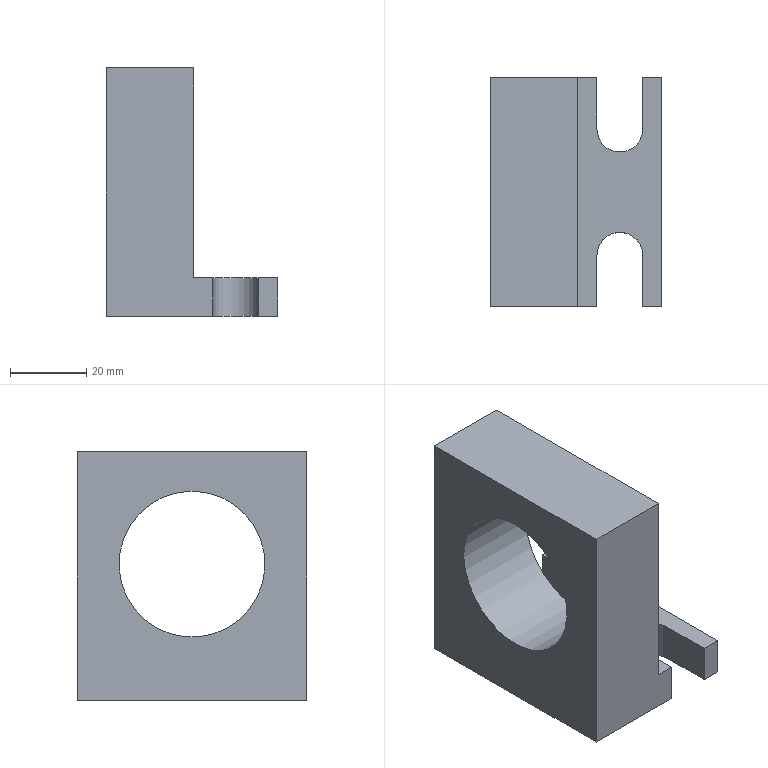Part | NX | features solid 2 | 1 solid | 17 faces | box 45 x 60 x 65 mm | volume 72169 mm3 | plane 14 | cylinder 3 | commonest cylinder face diameters 12 x2 38.2 x1
STEP:
#1=CARTESIAN_POINT('',(350.,-180.,-430.3));
#2=VERTEX_POINT('',#1);
#3=CARTESIAN_POINT('',(350.,-180.,-449.4));
#4=DIRECTION('',(-1.,0.,0.));
#5=DIRECTION('',(0.,0.,1.));
#6=AXIS2_PLACEMENT_3D('',#3,#4,#5);
#7=CIRCLE('',#6,19.1);
#8=EDGE_CURVE('',#2,#2,#7,.T.);
#9=ORIENTED_EDGE('',*,*,#8,.F.);
#10=EDGE_LOOP('',(#9));
#11=FACE_BOUND('',#10,.T.);
#12=CARTESIAN_POINT('',(350.,-150.,-420.));
#13=VERTEX_POINT('',#12);
#14=CARTESIAN_POINT('',(350.,-150.,-485.));
#15=VERTEX_POINT('',#14);
#16=CARTESIAN_POINT('',(350.,-150.,-417.4));
#17=DIRECTION('',(0.,0.,-1.));
#18=VECTOR('',#17,1000.);
#19=LINE('',#16,#18);
#20=EDGE_CURVE('',#13,#15,#19,.T.);
#21=ORIENTED_EDGE('',*,*,#20,.T.);
#22=CARTESIAN_POINT('',(350.,-210.,-485.));
#23=VERTEX_POINT('',#22);
#24=CARTESIAN_POINT('',(350.,-212.5,-485.));
#25=DIRECTION('',(0.,-1.,0.));
#26=VECTOR('',#25,1000.);
#27=LINE('',#24,#26);
#28=EDGE_CURVE('',#23,#15,#27,.F.);
#29=ORIENTED_EDGE('',*,*,#28,.F.);
#30=CARTESIAN_POINT('',(350.,-210.,-420.));
#31=VERTEX_POINT('',#30);
#32=CARTESIAN_POINT('',(350.,-210.,-417.4));
#33=DIRECTION('',(0.,0.,1.));
#34=VECTOR('',#33,1000.);
#35=LINE('',#32,#34);
#36=EDGE_CURVE('',#31,#23,#35,.F.);
#37=ORIENTED_EDGE('',*,*,#36,.F.);
#38=CARTESIAN_POINT('',(350.,-212.5,-420.));
#39=DIRECTION('',(0.,1.,0.));
#40=VECTOR('',#39,1000.);
#41=LINE('',#38,#40);
#42=EDGE_CURVE('',#31,#13,#41,.T.);
#43=ORIENTED_EDGE('',*,*,#42,.T.);
#44=EDGE_LOOP('',(#21,#29,#37,#43));
#45=FACE_BOUND('',#44,.T.);
#46=CARTESIAN_POINT('',(350.,-212.5,-417.4));
#47=DIRECTION('',(-1.,0.,0.));
#48=DIRECTION('',(0.,0.,-1.));
#49=AXIS2_PLACEMENT_3D('',#46,#47,#48);
#50=PLANE('',#49);
#51=ADVANCED_FACE('',(#11,#45),#50,.T.);
#52=CARTESIAN_POINT('',(395.,-210.,-485.));
#53=VERTEX_POINT('',#52);
#54=CARTESIAN_POINT('',(395.,-150.,-485.));
#55=VERTEX_POINT('',#54);
#56=CARTESIAN_POINT('',(395.,-212.5,-485.));
#57=DIRECTION('',(0.,-1.,0.));
#58=VECTOR('',#57,1000.);
#59=LINE('',#56,#58);
#60=EDGE_CURVE('',#53,#55,#59,.F.);
#61=ORIENTED_EDGE('',*,*,#60,.T.);
#62=CARTESIAN_POINT('',(395.,-150.,-475.));
#63=VERTEX_POINT('',#62);
#64=CARTESIAN_POINT('',(395.,-150.,-417.4));
#65=DIRECTION('',(0.,0.,-1.));
#66=VECTOR('',#65,1000.);
#67=LINE('',#64,#66);
#68=EDGE_CURVE('',#63,#55,#67,.T.);
#69=ORIENTED_EDGE('',*,*,#68,.F.);
#70=CARTESIAN_POINT('',(395.,-210.,-475.));
#71=VERTEX_POINT('',#70);
#72=CARTESIAN_POINT('',(395.,-212.5,-475.));
#73=DIRECTION('',(0.,1.,0.));
#74=VECTOR('',#73,1000.);
#75=LINE('',#72,#74);
#76=EDGE_CURVE('',#71,#63,#75,.T.);
#77=ORIENTED_EDGE('',*,*,#76,.F.);
#78=CARTESIAN_POINT('',(395.,-210.,-487.4));
#79=DIRECTION('',(0.,0.,1.));
#80=VECTOR('',#79,1000.);
#81=LINE('',#78,#80);
#82=EDGE_CURVE('',#71,#53,#81,.F.);
#83=ORIENTED_EDGE('',*,*,#82,.T.);
#84=EDGE_LOOP('',(#61,#69,#77,#83));
#85=FACE_BOUND('',#84,.T.);
#86=CARTESIAN_POINT('',(395.,-212.5,-487.4));
#87=DIRECTION('',(-1.,0.,0.));
#88=DIRECTION('',(0.,1.,0.));
#89=AXIS2_PLACEMENT_3D('',#86,#87,#88);
#90=PLANE('',#89);
#91=ADVANCED_FACE('',(#85),#90,.F.);
#92=CARTESIAN_POINT('',(378.,-210.,-485.));
#93=VERTEX_POINT('',#92);
#94=CARTESIAN_POINT('',(378.,-210.,-475.));
#95=VERTEX_POINT('',#94);
#96=CARTESIAN_POINT('',(378.,-210.,-524.4));
#97=DIRECTION('',(0.,0.,-1.));
#98=VECTOR('',#97,1000.);
#99=LINE('',#96,#98);
#100=EDGE_CURVE('',#93,#95,#99,.F.);
#101=ORIENTED_EDGE('',*,*,#100,.T.);
#102=CARTESIAN_POINT('',(373.,-210.,-475.));
#103=VERTEX_POINT('',#102);
#104=CARTESIAN_POINT('',(373.,-210.,-475.));
#105=DIRECTION('',(-1.,0.,0.));
#106=VECTOR('',#105,1000.);
#107=LINE('',#104,#106);
#108=EDGE_CURVE('',#103,#95,#107,.F.);
#109=ORIENTED_EDGE('',*,*,#108,.F.);
#110=CARTESIAN_POINT('',(373.,-210.,-420.));
#111=VERTEX_POINT('',#110);
#112=CARTESIAN_POINT('',(373.,-210.,-417.4));
#113=DIRECTION('',(0.,0.,1.));
#114=VECTOR('',#113,1000.);
#115=LINE('',#112,#114);
#116=EDGE_CURVE('',#111,#103,#115,.F.);
#117=ORIENTED_EDGE('',*,*,#116,.F.);
#118=CARTESIAN_POINT('',(373.,-210.,-420.));
#119=DIRECTION('',(-1.,0.,0.));
#120=VECTOR('',#119,1000.);
#121=LINE('',#118,#120);
#122=EDGE_CURVE('',#31,#111,#121,.F.);
#123=ORIENTED_EDGE('',*,*,#122,.F.);
#124=ORIENTED_EDGE('',*,*,#36,.T.);
#125=CARTESIAN_POINT('',(373.,-210.,-485.));
#126=DIRECTION('',(1.,0.,0.));
#127=VECTOR('',#126,1000.);
#128=LINE('',#125,#127);
#129=EDGE_CURVE('',#23,#93,#128,.T.);
#130=ORIENTED_EDGE('',*,*,#129,.T.);
#131=EDGE_LOOP('',(#101,#109,#117,#123,#124,#130));
#132=FACE_BOUND('',#131,.T.);
#133=CARTESIAN_POINT('',(373.,-210.,-417.4));
#134=DIRECTION('',(0.,-1.,0.));
#135=DIRECTION('',(0.,0.,-1.));
#136=AXIS2_PLACEMENT_3D('',#133,#134,#135);
#137=PLANE('',#136);
#138=ADVANCED_FACE('',(#132),#137,.T.);
#139=ORIENTED_EDGE('',*,*,#60,.F.);
#140=CARTESIAN_POINT('',(390.,-210.,-485.));
#141=VERTEX_POINT('',#140);
#142=CARTESIAN_POINT('',(373.,-210.,-485.));
#143=DIRECTION('',(1.,0.,0.));
#144=VECTOR('',#143,1000.);
#145=LINE('',#142,#144);
#146=EDGE_CURVE('',#141,#53,#145,.T.);
#147=ORIENTED_EDGE('',*,*,#146,.F.);
#148=CARTESIAN_POINT('',(390.,-196.5,-485.));
#149=VERTEX_POINT('',#148);
#150=CARTESIAN_POINT('',(390.,-212.5,-485.));
#151=DIRECTION('',(0.,1.,0.));
#152=VECTOR('',#151,1000.);
#153=LINE('',#150,#152);
#154=EDGE_CURVE('',#149,#141,#153,.F.);
#155=ORIENTED_EDGE('',*,*,#154,.F.);
#156=CARTESIAN_POINT('',(378.,-196.5,-485.));
#157=VERTEX_POINT('',#156);
#158=CARTESIAN_POINT('',(384.,-196.5,-485.));
#159=DIRECTION('',(0.,0.,1.));
#160=DIRECTION('',(0.,1.,0.));
#161=AXIS2_PLACEMENT_3D('',#158,#159,#160);
#162=CIRCLE('',#161,6.);
#163=EDGE_CURVE('',#157,#149,#162,.F.);
#164=ORIENTED_EDGE('',*,*,#163,.F.);
#165=CARTESIAN_POINT('',(378.,-212.5,-485.));
#166=DIRECTION('',(0.,1.,0.));
#167=VECTOR('',#166,1000.);
#168=LINE('',#165,#167);
#169=EDGE_CURVE('',#157,#93,#168,.F.);
#170=ORIENTED_EDGE('',*,*,#169,.T.);
#171=ORIENTED_EDGE('',*,*,#129,.F.);
#172=ORIENTED_EDGE('',*,*,#28,.T.);
#173=CARTESIAN_POINT('',(378.,-150.,-485.));
#174=VERTEX_POINT('',#173);
#175=CARTESIAN_POINT('',(373.,-150.,-485.));
#176=DIRECTION('',(-1.,0.,0.));
#177=VECTOR('',#176,1000.);
#178=LINE('',#175,#177);
#179=EDGE_CURVE('',#15,#174,#178,.F.);
#180=ORIENTED_EDGE('',*,*,#179,.T.);
#181=CARTESIAN_POINT('',(378.,-163.5,-485.));
#182=VERTEX_POINT('',#181);
#183=CARTESIAN_POINT('',(378.,-212.5,-485.));
#184=DIRECTION('',(0.,-1.,0.));
#185=VECTOR('',#184,1000.);
#186=LINE('',#183,#185);
#187=EDGE_CURVE('',#182,#174,#186,.F.);
#188=ORIENTED_EDGE('',*,*,#187,.F.);
#189=CARTESIAN_POINT('',(390.,-163.5,-485.));
#190=VERTEX_POINT('',#189);
#191=CARTESIAN_POINT('',(384.,-163.5,-485.));
#192=DIRECTION('',(0.,0.,1.));
#193=DIRECTION('',(0.,1.,0.));
#194=AXIS2_PLACEMENT_3D('',#191,#192,#193);
#195=CIRCLE('',#194,6.);
#196=EDGE_CURVE('',#190,#182,#195,.F.);
#197=ORIENTED_EDGE('',*,*,#196,.F.);
#198=CARTESIAN_POINT('',(390.,-150.,-485.));
#199=VERTEX_POINT('',#198);
#200=CARTESIAN_POINT('',(390.,-212.5,-485.));
#201=DIRECTION('',(0.,-1.,0.));
#202=VECTOR('',#201,1000.);
#203=LINE('',#200,#202);
#204=EDGE_CURVE('',#190,#199,#203,.F.);
#205=ORIENTED_EDGE('',*,*,#204,.T.);
#206=CARTESIAN_POINT('',(373.,-150.,-485.));
#207=DIRECTION('',(-1.,0.,0.));
#208=VECTOR('',#207,1000.);
#209=LINE('',#206,#208);
#210=EDGE_CURVE('',#199,#55,#209,.F.);
#211=ORIENTED_EDGE('',*,*,#210,.T.);
#212=EDGE_LOOP('',(#139,#147,#155,#164,#170,#171,#172,#180,#188,#197,#205,#211));
#213=FACE_BOUND('',#212,.T.);
#214=CARTESIAN_POINT('',(373.,-212.5,-485.));
#215=DIRECTION('',(0.,0.,-1.));
#216=DIRECTION('',(0.,1.,0.));
#217=AXIS2_PLACEMENT_3D('',#214,#215,#216);
#218=PLANE('',#217);
#219=ADVANCED_FACE('',(#213),#218,.T.);
#220=CARTESIAN_POINT('',(378.,-196.5,-475.));
#221=VERTEX_POINT('',#220);
#222=CARTESIAN_POINT('',(390.,-196.5,-475.));
#223=VERTEX_POINT('',#222);
#224=CARTESIAN_POINT('',(384.,-196.5,-475.));
#225=DIRECTION('',(0.,0.,-1.));
#226=DIRECTION('',(0.,-1.,0.));
#227=AXIS2_PLACEMENT_3D('',#224,#225,#226);
#228=CIRCLE('',#227,6.);
#229=EDGE_CURVE('',#221,#223,#228,.T.);
#230=ORIENTED_EDGE('',*,*,#229,.T.);
#231=CARTESIAN_POINT('',(390.,-210.,-475.));
#232=VERTEX_POINT('',#231);
#233=CARTESIAN_POINT('',(390.,-212.5,-475.));
#234=DIRECTION('',(0.,-1.,0.));
#235=VECTOR('',#234,1000.);
#236=LINE('',#233,#235);
#237=EDGE_CURVE('',#223,#232,#236,.T.);
#238=ORIENTED_EDGE('',*,*,#237,.T.);
#239=CARTESIAN_POINT('',(373.,-210.,-475.));
#240=DIRECTION('',(-1.,0.,0.));
#241=VECTOR('',#240,1000.);
#242=LINE('',#239,#241);
#243=EDGE_CURVE('',#232,#71,#242,.F.);
#244=ORIENTED_EDGE('',*,*,#243,.T.);
#245=ORIENTED_EDGE('',*,*,#76,.T.);
#246=CARTESIAN_POINT('',(390.,-150.,-475.));
#247=VERTEX_POINT('',#246);
#248=CARTESIAN_POINT('',(373.,-150.,-475.));
#249=DIRECTION('',(1.,0.,0.));
#250=VECTOR('',#249,1000.);
#251=LINE('',#248,#250);
#252=EDGE_CURVE('',#247,#63,#251,.T.);
#253=ORIENTED_EDGE('',*,*,#252,.F.);
#254=CARTESIAN_POINT('',(390.,-163.5,-475.));
#255=VERTEX_POINT('',#254);
#256=CARTESIAN_POINT('',(390.,-212.5,-475.));
#257=DIRECTION('',(0.,1.,0.));
#258=VECTOR('',#257,1000.);
#259=LINE('',#256,#258);
#260=EDGE_CURVE('',#255,#247,#259,.T.);
#261=ORIENTED_EDGE('',*,*,#260,.F.);
#262=CARTESIAN_POINT('',(378.,-163.5,-475.));
#263=VERTEX_POINT('',#262);
#264=CARTESIAN_POINT('',(384.,-163.5,-475.));
#265=DIRECTION('',(0.,0.,-1.));
#266=DIRECTION('',(0.,-1.,0.));
#267=AXIS2_PLACEMENT_3D('',#264,#265,#266);
#268=CIRCLE('',#267,6.);
#269=EDGE_CURVE('',#255,#263,#268,.T.);
#270=ORIENTED_EDGE('',*,*,#269,.T.);
#271=CARTESIAN_POINT('',(378.,-150.,-475.));
#272=VERTEX_POINT('',#271);
#273=CARTESIAN_POINT('',(378.,-212.5,-475.));
#274=DIRECTION('',(0.,1.,0.));
#275=VECTOR('',#274,1000.);
#276=LINE('',#273,#275);
#277=EDGE_CURVE('',#263,#272,#276,.T.);
#278=ORIENTED_EDGE('',*,*,#277,.T.);
#279=CARTESIAN_POINT('',(373.,-150.,-475.));
#280=VERTEX_POINT('',#279);
#281=CARTESIAN_POINT('',(373.,-150.,-475.));
#282=DIRECTION('',(1.,0.,0.));
#283=VECTOR('',#282,1000.);
#284=LINE('',#281,#283);
#285=EDGE_CURVE('',#280,#272,#284,.T.);
#286=ORIENTED_EDGE('',*,*,#285,.F.);
#287=CARTESIAN_POINT('',(373.,-212.5,-475.));
#288=DIRECTION('',(0.,1.,0.));
#289=VECTOR('',#288,1000.);
#290=LINE('',#287,#289);
#291=EDGE_CURVE('',#103,#280,#290,.T.);
#292=ORIENTED_EDGE('',*,*,#291,.F.);
#293=ORIENTED_EDGE('',*,*,#108,.T.);
#294=CARTESIAN_POINT('',(378.,-212.5,-475.));
#295=DIRECTION('',(0.,-1.,0.));
#296=VECTOR('',#295,1000.);
#297=LINE('',#294,#296);
#298=EDGE_CURVE('',#221,#95,#297,.T.);
#299=ORIENTED_EDGE('',*,*,#298,.F.);
#300=EDGE_LOOP('',(#230,#238,#244,#245,#253,#261,#270,#278,#286,#292,#293,#299));
#301=FACE_BOUND('',#300,.T.);
#302=CARTESIAN_POINT('',(373.,-212.5,-475.));
#303=DIRECTION('',(0.,0.,1.));
#304=DIRECTION('',(-1.,0.,0.));
#305=AXIS2_PLACEMENT_3D('',#302,#303,#304);
#306=PLANE('',#305);
#307=ADVANCED_FACE('',(#301),#306,.T.);
#308=CARTESIAN_POINT('',(390.,-150.,-524.4));
#309=DIRECTION('',(0.,0.,1.));
#310=VECTOR('',#309,1000.);
#311=LINE('',#308,#310);
#312=EDGE_CURVE('',#199,#247,#311,.T.);
#313=ORIENTED_EDGE('',*,*,#312,.T.);
#314=ORIENTED_EDGE('',*,*,#252,.T.);
#315=ORIENTED_EDGE('',*,*,#68,.T.);
#316=ORIENTED_EDGE('',*,*,#210,.F.);
#317=EDGE_LOOP('',(#313,#314,#315,#316));
#318=FACE_BOUND('',#317,.T.);
#319=CARTESIAN_POINT('',(373.,-150.,-417.4));
#320=DIRECTION('',(0.,-1.,0.));
#321=DIRECTION('',(0.,0.,-1.));
#322=AXIS2_PLACEMENT_3D('',#319,#320,#321);
#323=PLANE('',#322);
#324=ADVANCED_FACE('',(#318),#323,.F.);
#325=ORIENTED_EDGE('',*,*,#116,.T.);
#326=ORIENTED_EDGE('',*,*,#291,.T.);
#327=CARTESIAN_POINT('',(373.,-150.,-420.));
#328=VERTEX_POINT('',#327);
#329=CARTESIAN_POINT('',(373.,-150.,-417.4));
#330=DIRECTION('',(0.,0.,-1.));
#331=VECTOR('',#330,1000.);
#332=LINE('',#329,#331);
#333=EDGE_CURVE('',#328,#280,#332,.T.);
#334=ORIENTED_EDGE('',*,*,#333,.F.);
#335=CARTESIAN_POINT('',(373.,-212.5,-420.));
#336=DIRECTION('',(0.,1.,0.));
#337=VECTOR('',#336,1000.);
#338=LINE('',#335,#337);
#339=EDGE_CURVE('',#111,#328,#338,.T.);
#340=ORIENTED_EDGE('',*,*,#339,.F.);
#341=EDGE_LOOP('',(#325,#326,#334,#340));
#342=FACE_BOUND('',#341,.T.);
#343=CARTESIAN_POINT('',(373.,-180.,-430.3));
#344=VERTEX_POINT('',#343);
#345=CARTESIAN_POINT('',(373.,-180.,-449.4));
#346=DIRECTION('',(-1.,0.,0.));
#347=DIRECTION('',(0.,0.,1.));
#348=AXIS2_PLACEMENT_3D('',#345,#346,#347);
#349=CIRCLE('',#348,19.1);
#350=EDGE_CURVE('',#344,#344,#349,.F.);
#351=ORIENTED_EDGE('',*,*,#350,.F.);
#352=EDGE_LOOP('',(#351));
#353=FACE_BOUND('',#352,.T.);
#354=CARTESIAN_POINT('',(373.,-212.5,-417.4));
#355=DIRECTION('',(-1.,0.,0.));
#356=DIRECTION('',(0.,0.,-1.));
#357=AXIS2_PLACEMENT_3D('',#354,#355,#356);
#358=PLANE('',#357);
#359=ADVANCED_FACE('',(#342,#353),#358,.F.);
#360=ORIENTED_EDGE('',*,*,#146,.T.);
#361=ORIENTED_EDGE('',*,*,#82,.F.);
#362=ORIENTED_EDGE('',*,*,#243,.F.);
#363=CARTESIAN_POINT('',(390.,-210.,-524.4));
#364=DIRECTION('',(0.,0.,-1.));
#365=VECTOR('',#364,1000.);
#366=LINE('',#363,#365);
#367=EDGE_CURVE('',#141,#232,#366,.F.);
#368=ORIENTED_EDGE('',*,*,#367,.F.);
#369=EDGE_LOOP('',(#360,#361,#362,#368));
#370=FACE_BOUND('',#369,.T.);
#371=CARTESIAN_POINT('',(373.,-210.,-417.4));
#372=DIRECTION('',(0.,-1.,0.));
#373=DIRECTION('',(0.,0.,-1.));
#374=AXIS2_PLACEMENT_3D('',#371,#372,#373);
#375=PLANE('',#374);
#376=ADVANCED_FACE('',(#370),#375,.T.);
#377=ORIENTED_EDGE('',*,*,#179,.F.);
#378=ORIENTED_EDGE('',*,*,#20,.F.);
#379=CARTESIAN_POINT('',(373.,-150.,-420.));
#380=DIRECTION('',(1.,0.,0.));
#381=VECTOR('',#380,1000.);
#382=LINE('',#379,#381);
#383=EDGE_CURVE('',#13,#328,#382,.T.);
#384=ORIENTED_EDGE('',*,*,#383,.T.);
#385=ORIENTED_EDGE('',*,*,#333,.T.);
#386=ORIENTED_EDGE('',*,*,#285,.T.);
#387=CARTESIAN_POINT('',(378.,-150.,-524.4));
#388=DIRECTION('',(0.,0.,1.));
#389=VECTOR('',#388,1000.);
#390=LINE('',#387,#389);
#391=EDGE_CURVE('',#174,#272,#390,.T.);
#392=ORIENTED_EDGE('',*,*,#391,.F.);
#393=EDGE_LOOP('',(#377,#378,#384,#385,#386,#392));
#394=FACE_BOUND('',#393,.T.);
#395=CARTESIAN_POINT('',(373.,-150.,-417.4));
#396=DIRECTION('',(0.,-1.,0.));
#397=DIRECTION('',(0.,0.,-1.));
#398=AXIS2_PLACEMENT_3D('',#395,#396,#397);
#399=PLANE('',#398);
#400=ADVANCED_FACE('',(#394),#399,.F.);
#401=ORIENTED_EDGE('',*,*,#42,.F.);
#402=ORIENTED_EDGE('',*,*,#122,.T.);
#403=ORIENTED_EDGE('',*,*,#339,.T.);
#404=ORIENTED_EDGE('',*,*,#383,.F.);
#405=EDGE_LOOP('',(#401,#402,#403,#404));
#406=FACE_BOUND('',#405,.T.);
#407=CARTESIAN_POINT('',(373.,-212.5,-420.));
#408=DIRECTION('',(0.,0.,-1.));
#409=DIRECTION('',(0.,1.,0.));
#410=AXIS2_PLACEMENT_3D('',#407,#408,#409);
#411=PLANE('',#410);
#412=ADVANCED_FACE('',(#406),#411,.F.);
#413=ORIENTED_EDGE('',*,*,#8,.T.);
#414=EDGE_LOOP('',(#413));
#415=FACE_BOUND('',#414,.T.);
#416=ORIENTED_EDGE('',*,*,#350,.T.);
#417=EDGE_LOOP('',(#416));
#418=FACE_BOUND('',#417,.T.);
#419=CARTESIAN_POINT('',(293.,-180.,-449.4));
#420=DIRECTION('',(1.,0.,0.));
#421=DIRECTION('',(0.,0.,1.));
#422=AXIS2_PLACEMENT_3D('',#419,#420,#421);
#423=CYLINDRICAL_SURFACE('',#422,19.1);
#424=ADVANCED_FACE('',(#415,#418),#423,.F.);
#425=CARTESIAN_POINT('',(378.,-163.5,-524.4));
#426=DIRECTION('',(0.,0.,1.));
#427=VECTOR('',#426,1000.);
#428=LINE('',#425,#427);
#429=EDGE_CURVE('',#182,#263,#428,.T.);
#430=ORIENTED_EDGE('',*,*,#429,.F.);
#431=ORIENTED_EDGE('',*,*,#187,.T.);
#432=ORIENTED_EDGE('',*,*,#391,.T.);
#433=ORIENTED_EDGE('',*,*,#277,.F.);
#434=EDGE_LOOP('',(#430,#431,#432,#433));
#435=FACE_BOUND('',#434,.T.);
#436=CARTESIAN_POINT('',(378.,-163.5,-524.4));
#437=DIRECTION('',(-1.,0.,0.));
#438=DIRECTION('',(0.,0.,-1.));
#439=AXIS2_PLACEMENT_3D('',#436,#437,#438);
#440=PLANE('',#439);
#441=ADVANCED_FACE('',(#435),#440,.F.);
#442=ORIENTED_EDGE('',*,*,#204,.F.);
#443=CARTESIAN_POINT('',(390.,-163.5,-524.4));
#444=DIRECTION('',(0.,0.,1.));
#445=VECTOR('',#444,1000.);
#446=LINE('',#443,#445);
#447=EDGE_CURVE('',#190,#255,#446,.T.);
#448=ORIENTED_EDGE('',*,*,#447,.T.);
#449=ORIENTED_EDGE('',*,*,#260,.T.);
#450=ORIENTED_EDGE('',*,*,#312,.F.);
#451=EDGE_LOOP('',(#442,#448,#449,#450));
#452=FACE_BOUND('',#451,.T.);
#453=CARTESIAN_POINT('',(390.,-163.5,-524.4));
#454=DIRECTION('',(-1.,0.,0.));
#455=DIRECTION('',(0.,0.,-1.));
#456=AXIS2_PLACEMENT_3D('',#453,#454,#455);
#457=PLANE('',#456);
#458=ADVANCED_FACE('',(#452),#457,.T.);
#459=ORIENTED_EDGE('',*,*,#447,.F.);
#460=ORIENTED_EDGE('',*,*,#196,.T.);
#461=ORIENTED_EDGE('',*,*,#429,.T.);
#462=ORIENTED_EDGE('',*,*,#269,.F.);
#463=EDGE_LOOP('',(#459,#460,#461,#462));
#464=FACE_BOUND('',#463,.T.);
#465=CARTESIAN_POINT('',(384.,-163.5,-524.4));
#466=DIRECTION('',(0.,0.,1.));
#467=DIRECTION('',(-1.,0.,0.));
#468=AXIS2_PLACEMENT_3D('',#465,#466,#467);
#469=CYLINDRICAL_SURFACE('',#468,6.);
#470=ADVANCED_FACE('',(#464),#469,.F.);
#471=ORIENTED_EDGE('',*,*,#169,.F.);
#472=CARTESIAN_POINT('',(378.,-196.5,-524.4));
#473=DIRECTION('',(0.,0.,1.));
#474=VECTOR('',#473,1000.);
#475=LINE('',#472,#474);
#476=EDGE_CURVE('',#157,#221,#475,.T.);
#477=ORIENTED_EDGE('',*,*,#476,.T.);
#478=ORIENTED_EDGE('',*,*,#298,.T.);
#479=ORIENTED_EDGE('',*,*,#100,.F.);
#480=EDGE_LOOP('',(#471,#477,#478,#479));
#481=FACE_BOUND('',#480,.T.);
#482=CARTESIAN_POINT('',(378.,-196.5,-524.4));
#483=DIRECTION('',(1.,0.,0.));
#484=DIRECTION('',(0.,0.,1.));
#485=AXIS2_PLACEMENT_3D('',#482,#483,#484);
#486=PLANE('',#485);
#487=ADVANCED_FACE('',(#481),#486,.T.);
#488=ORIENTED_EDGE('',*,*,#476,.F.);
#489=ORIENTED_EDGE('',*,*,#163,.T.);
#490=CARTESIAN_POINT('',(390.,-196.5,-524.4));
#491=DIRECTION('',(0.,0.,1.));
#492=VECTOR('',#491,1000.);
#493=LINE('',#490,#492);
#494=EDGE_CURVE('',#149,#223,#493,.T.);
#495=ORIENTED_EDGE('',*,*,#494,.T.);
#496=ORIENTED_EDGE('',*,*,#229,.F.);
#497=EDGE_LOOP('',(#488,#489,#495,#496));
#498=FACE_BOUND('',#497,.T.);
#499=CARTESIAN_POINT('',(384.,-196.5,-524.4));
#500=DIRECTION('',(0.,0.,1.));
#501=DIRECTION('',(-1.,0.,0.));
#502=AXIS2_PLACEMENT_3D('',#499,#500,#501);
#503=CYLINDRICAL_SURFACE('',#502,6.);
#504=ADVANCED_FACE('',(#498),#503,.F.);
#505=ORIENTED_EDGE('',*,*,#494,.F.);
#506=ORIENTED_EDGE('',*,*,#154,.T.);
#507=ORIENTED_EDGE('',*,*,#367,.T.);
#508=ORIENTED_EDGE('',*,*,#237,.F.);
#509=EDGE_LOOP('',(#505,#506,#507,#508));
#510=FACE_BOUND('',#509,.T.);
#511=CARTESIAN_POINT('',(390.,-196.5,-524.4));
#512=DIRECTION('',(1.,0.,0.));
#513=DIRECTION('',(0.,0.,1.));
#514=AXIS2_PLACEMENT_3D('',#511,#512,#513);
#515=PLANE('',#514);
#516=ADVANCED_FACE('',(#510),#515,.F.);
#517=CLOSED_SHELL('',(#51,#91,#138,#219,#307,#324,#359,#376,#400,#412,#424,#441,#458,#470,#487,#504,#516));
#518=MANIFOLD_SOLID_BREP('',#517);
#519=(LENGTH_UNIT()NAMED_UNIT(*)SI_UNIT(.MILLI.,.METRE.));
#520=UNCERTAINTY_MEASURE_WITH_UNIT(LENGTH_MEASURE(0.00001),#519,'','');
#521=(NAMED_UNIT(*)PLANE_ANGLE_UNIT()SI_UNIT($,.RADIAN.));
#522=(NAMED_UNIT(*)SI_UNIT($,.STERADIAN.)SOLID_ANGLE_UNIT());
#523=(GEOMETRIC_REPRESENTATION_CONTEXT(3)GLOBAL_UNCERTAINTY_ASSIGNED_CONTEXT((#520))GLOBAL_UNIT_ASSIGNED_CONTEXT((#519,#521,#522))REPRESENTATION_CONTEXT('',''));
#524=ADVANCED_BREP_SHAPE_REPRESENTATION('',(#518),#523);